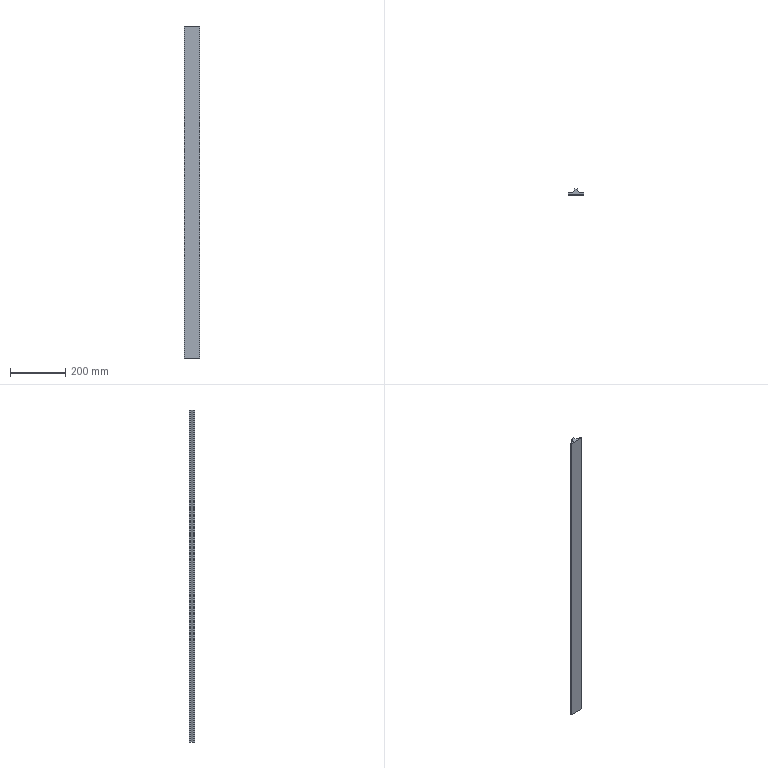Part | STEP file | SOPORTE RIEL 25mm | 1 solid | 13 faces | box 55 x 21.275 x 1200 mm | volume 648615 mm3 | plane 13
STEP:
#1=CARTESIAN_POINT('',(27.5,0.,-600.));
#2=VERTEX_POINT('',#1);
#3=CARTESIAN_POINT('',(27.5,6.,-600.));
#4=VERTEX_POINT('',#3);
#5=CARTESIAN_POINT('',(27.5,0.,-600.));
#6=DIRECTION('',(0.,1.,0.));
#7=VECTOR('',#6,1000.);
#8=LINE('',#5,#7);
#9=EDGE_CURVE('',#2,#4,#8,.T.);
#10=ORIENTED_EDGE('',*,*,#9,.T.);
#11=CARTESIAN_POINT('',(27.5,6.,600.));
#12=VERTEX_POINT('',#11);
#13=CARTESIAN_POINT('',(27.5,6.,600.));
#14=DIRECTION('',(0.,0.,-1.));
#15=VECTOR('',#14,1000.);
#16=LINE('',#13,#15);
#17=EDGE_CURVE('',#12,#4,#16,.T.);
#18=ORIENTED_EDGE('',*,*,#17,.F.);
#19=CARTESIAN_POINT('',(27.5,0.,600.));
#20=VERTEX_POINT('',#19);
#21=CARTESIAN_POINT('',(27.5,0.,600.));
#22=DIRECTION('',(0.,1.,0.));
#23=VECTOR('',#22,1000.);
#24=LINE('',#21,#23);
#25=EDGE_CURVE('',#20,#12,#24,.T.);
#26=ORIENTED_EDGE('',*,*,#25,.F.);
#27=CARTESIAN_POINT('',(27.5,0.,600.));
#28=DIRECTION('',(0.,0.,-1.));
#29=VECTOR('',#28,1000.);
#30=LINE('',#27,#29);
#31=EDGE_CURVE('',#20,#2,#30,.T.);
#32=ORIENTED_EDGE('',*,*,#31,.T.);
#33=EDGE_LOOP('',(#10,#18,#26,#32));
#34=FACE_OUTER_BOUND('',#33,.T.);
#35=CARTESIAN_POINT('',(27.5,0.,600.));
#36=DIRECTION('',(-1.,0.,0.));
#37=DIRECTION('',(0.,0.,1.));
#38=AXIS2_PLACEMENT_3D('',#35,#36,#37);
#39=PLANE('',#38);
#40=ADVANCED_FACE('',(#34),#39,.F.);
#41=CARTESIAN_POINT('',(11.,6.,-600.));
#42=VERTEX_POINT('',#41);
#43=CARTESIAN_POINT('',(27.5,6.,-600.));
#44=DIRECTION('',(-1.,0.,0.));
#45=VECTOR('',#44,1000.);
#46=LINE('',#43,#45);
#47=EDGE_CURVE('',#4,#42,#46,.T.);
#48=ORIENTED_EDGE('',*,*,#47,.T.);
#49=CARTESIAN_POINT('',(11.,6.,600.));
#50=VERTEX_POINT('',#49);
#51=CARTESIAN_POINT('',(11.,6.,600.));
#52=DIRECTION('',(0.,0.,-1.));
#53=VECTOR('',#52,1000.);
#54=LINE('',#51,#53);
#55=EDGE_CURVE('',#50,#42,#54,.T.);
#56=ORIENTED_EDGE('',*,*,#55,.F.);
#57=CARTESIAN_POINT('',(27.5,6.,600.));
#58=DIRECTION('',(-1.,0.,0.));
#59=VECTOR('',#58,1000.);
#60=LINE('',#57,#59);
#61=EDGE_CURVE('',#12,#50,#60,.T.);
#62=ORIENTED_EDGE('',*,*,#61,.F.);
#63=ORIENTED_EDGE('',*,*,#17,.T.);
#64=EDGE_LOOP('',(#48,#56,#62,#63));
#65=FACE_OUTER_BOUND('',#64,.T.);
#66=CARTESIAN_POINT('',(27.5,6.,600.));
#67=DIRECTION('',(0.,-1.,0.));
#68=DIRECTION('',(0.,0.,-1.));
#69=AXIS2_PLACEMENT_3D('',#66,#67,#68);
#70=PLANE('',#69);
#71=ADVANCED_FACE('',(#65),#70,.F.);
#72=CARTESIAN_POINT('',(5.5,15.,-600.));
#73=VERTEX_POINT('',#72);
#74=CARTESIAN_POINT('',(11.,6.,-600.));
#75=DIRECTION('',(-0.5215,0.8533,0.));
#76=VECTOR('',#75,1000.);
#77=LINE('',#74,#76);
#78=EDGE_CURVE('',#42,#73,#77,.T.);
#79=ORIENTED_EDGE('',*,*,#78,.T.);
#80=CARTESIAN_POINT('',(5.5,15.,600.));
#81=VERTEX_POINT('',#80);
#82=CARTESIAN_POINT('',(5.5,15.,600.));
#83=DIRECTION('',(0.,0.,-1.));
#84=VECTOR('',#83,1000.);
#85=LINE('',#82,#84);
#86=EDGE_CURVE('',#81,#73,#85,.T.);
#87=ORIENTED_EDGE('',*,*,#86,.F.);
#88=CARTESIAN_POINT('',(11.,6.,600.));
#89=DIRECTION('',(-0.5215,0.8533,0.));
#90=VECTOR('',#89,1000.);
#91=LINE('',#88,#90);
#92=EDGE_CURVE('',#50,#81,#91,.T.);
#93=ORIENTED_EDGE('',*,*,#92,.F.);
#94=ORIENTED_EDGE('',*,*,#55,.T.);
#95=EDGE_LOOP('',(#79,#87,#93,#94));
#96=FACE_OUTER_BOUND('',#95,.T.);
#97=CARTESIAN_POINT('',(11.,6.,600.));
#98=DIRECTION('',(-0.8533,-0.5215,0.));
#99=DIRECTION('',(0.5215,-0.8533,0.));
#100=AXIS2_PLACEMENT_3D('',#97,#98,#99);
#101=PLANE('',#100);
#102=ADVANCED_FACE('',(#96),#101,.F.);
#103=CARTESIAN_POINT('',(5.5,21.275,-600.));
#104=VERTEX_POINT('',#103);
#105=CARTESIAN_POINT('',(5.5,15.,-600.));
#106=DIRECTION('',(0.,1.,0.));
#107=VECTOR('',#106,1000.);
#108=LINE('',#105,#107);
#109=EDGE_CURVE('',#73,#104,#108,.T.);
#110=ORIENTED_EDGE('',*,*,#109,.T.);
#111=CARTESIAN_POINT('',(5.5,21.275,600.));
#112=VERTEX_POINT('',#111);
#113=CARTESIAN_POINT('',(5.5,21.275,600.));
#114=DIRECTION('',(0.,0.,-1.));
#115=VECTOR('',#114,1000.);
#116=LINE('',#113,#115);
#117=EDGE_CURVE('',#112,#104,#116,.T.);
#118=ORIENTED_EDGE('',*,*,#117,.F.);
#119=CARTESIAN_POINT('',(5.5,15.,600.));
#120=DIRECTION('',(0.,1.,0.));
#121=VECTOR('',#120,1000.);
#122=LINE('',#119,#121);
#123=EDGE_CURVE('',#81,#112,#122,.T.);
#124=ORIENTED_EDGE('',*,*,#123,.F.);
#125=ORIENTED_EDGE('',*,*,#86,.T.);
#126=EDGE_LOOP('',(#110,#118,#124,#125));
#127=FACE_OUTER_BOUND('',#126,.T.);
#128=CARTESIAN_POINT('',(5.5,15.,600.));
#129=DIRECTION('',(-1.,0.,0.));
#130=DIRECTION('',(0.,-1.,0.));
#131=AXIS2_PLACEMENT_3D('',#128,#129,#130);
#132=PLANE('',#131);
#133=ADVANCED_FACE('',(#127),#132,.F.);
#134=CARTESIAN_POINT('',(0.,20.,-600.));
#135=VERTEX_POINT('',#134);
#136=CARTESIAN_POINT('',(0.,20.,-600.));
#137=DIRECTION('',(-0.9742,-0.2258,0.));
#138=VECTOR('',#137,1000.);
#139=LINE('',#136,#138);
#140=EDGE_CURVE('',#104,#135,#139,.T.);
#141=ORIENTED_EDGE('',*,*,#140,.T.);
#142=CARTESIAN_POINT('',(0.,20.,600.));
#143=VERTEX_POINT('',#142);
#144=CARTESIAN_POINT('',(0.,20.,600.));
#145=DIRECTION('',(0.,0.,-1.));
#146=VECTOR('',#145,1000.);
#147=LINE('',#144,#146);
#148=EDGE_CURVE('',#143,#135,#147,.T.);
#149=ORIENTED_EDGE('',*,*,#148,.F.);
#150=CARTESIAN_POINT('',(0.,20.,600.));
#151=DIRECTION('',(-0.9742,-0.2258,0.));
#152=VECTOR('',#151,1000.);
#153=LINE('',#150,#152);
#154=EDGE_CURVE('',#112,#143,#153,.T.);
#155=ORIENTED_EDGE('',*,*,#154,.F.);
#156=ORIENTED_EDGE('',*,*,#117,.T.);
#157=EDGE_LOOP('',(#141,#149,#155,#156));
#158=FACE_OUTER_BOUND('',#157,.T.);
#159=CARTESIAN_POINT('',(0.,20.,600.));
#160=DIRECTION('',(0.2258,-0.9742,0.));
#161=DIRECTION('',(0.9742,0.2258,0.));
#162=AXIS2_PLACEMENT_3D('',#159,#160,#161);
#163=PLANE('',#162);
#164=ADVANCED_FACE('',(#158),#163,.F.);
#165=CARTESIAN_POINT('',(-5.5,21.275,-600.));
#166=VERTEX_POINT('',#165);
#167=CARTESIAN_POINT('',(-5.5,21.275,-600.));
#168=DIRECTION('',(-0.9742,0.2258,0.));
#169=VECTOR('',#168,1000.);
#170=LINE('',#167,#169);
#171=EDGE_CURVE('',#135,#166,#170,.T.);
#172=ORIENTED_EDGE('',*,*,#171,.T.);
#173=CARTESIAN_POINT('',(-5.5,21.275,600.));
#174=VERTEX_POINT('',#173);
#175=CARTESIAN_POINT('',(-5.5,21.275,600.));
#176=DIRECTION('',(0.,0.,-1.));
#177=VECTOR('',#176,1000.);
#178=LINE('',#175,#177);
#179=EDGE_CURVE('',#174,#166,#178,.T.);
#180=ORIENTED_EDGE('',*,*,#179,.F.);
#181=CARTESIAN_POINT('',(-5.5,21.275,600.));
#182=DIRECTION('',(-0.9742,0.2258,0.));
#183=VECTOR('',#182,1000.);
#184=LINE('',#181,#183);
#185=EDGE_CURVE('',#143,#174,#184,.T.);
#186=ORIENTED_EDGE('',*,*,#185,.F.);
#187=ORIENTED_EDGE('',*,*,#148,.T.);
#188=EDGE_LOOP('',(#172,#180,#186,#187));
#189=FACE_OUTER_BOUND('',#188,.T.);
#190=CARTESIAN_POINT('',(-5.5,21.275,600.));
#191=DIRECTION('',(-0.2258,-0.9742,0.));
#192=DIRECTION('',(0.9742,-0.2258,0.));
#193=AXIS2_PLACEMENT_3D('',#190,#191,#192);
#194=PLANE('',#193);
#195=ADVANCED_FACE('',(#189),#194,.F.);
#196=CARTESIAN_POINT('',(-5.5,15.,-600.));
#197=VERTEX_POINT('',#196);
#198=CARTESIAN_POINT('',(-5.5,15.,-600.));
#199=DIRECTION('',(0.,-1.,0.));
#200=VECTOR('',#199,1000.);
#201=LINE('',#198,#200);
#202=EDGE_CURVE('',#166,#197,#201,.T.);
#203=ORIENTED_EDGE('',*,*,#202,.T.);
#204=CARTESIAN_POINT('',(-5.5,15.,600.));
#205=VERTEX_POINT('',#204);
#206=CARTESIAN_POINT('',(-5.5,15.,600.));
#207=DIRECTION('',(0.,0.,-1.));
#208=VECTOR('',#207,1000.);
#209=LINE('',#206,#208);
#210=EDGE_CURVE('',#205,#197,#209,.T.);
#211=ORIENTED_EDGE('',*,*,#210,.F.);
#212=CARTESIAN_POINT('',(-5.5,15.,600.));
#213=DIRECTION('',(0.,-1.,0.));
#214=VECTOR('',#213,1000.);
#215=LINE('',#212,#214);
#216=EDGE_CURVE('',#174,#205,#215,.T.);
#217=ORIENTED_EDGE('',*,*,#216,.F.);
#218=ORIENTED_EDGE('',*,*,#179,.T.);
#219=EDGE_LOOP('',(#203,#211,#217,#218));
#220=FACE_OUTER_BOUND('',#219,.T.);
#221=CARTESIAN_POINT('',(-5.5,15.,600.));
#222=DIRECTION('',(1.,0.,0.));
#223=DIRECTION('',(0.,1.,0.));
#224=AXIS2_PLACEMENT_3D('',#221,#222,#223);
#225=PLANE('',#224);
#226=ADVANCED_FACE('',(#220),#225,.F.);
#227=CARTESIAN_POINT('',(-11.,6.,-600.));
#228=VERTEX_POINT('',#227);
#229=CARTESIAN_POINT('',(-11.,6.,-600.));
#230=DIRECTION('',(-0.5215,-0.8533,0.));
#231=VECTOR('',#230,1000.);
#232=LINE('',#229,#231);
#233=EDGE_CURVE('',#197,#228,#232,.T.);
#234=ORIENTED_EDGE('',*,*,#233,.T.);
#235=CARTESIAN_POINT('',(-11.,6.,600.));
#236=VERTEX_POINT('',#235);
#237=CARTESIAN_POINT('',(-11.,6.,600.));
#238=DIRECTION('',(0.,0.,-1.));
#239=VECTOR('',#238,1000.);
#240=LINE('',#237,#239);
#241=EDGE_CURVE('',#236,#228,#240,.T.);
#242=ORIENTED_EDGE('',*,*,#241,.F.);
#243=CARTESIAN_POINT('',(-11.,6.,600.));
#244=DIRECTION('',(-0.5215,-0.8533,0.));
#245=VECTOR('',#244,1000.);
#246=LINE('',#243,#245);
#247=EDGE_CURVE('',#205,#236,#246,.T.);
#248=ORIENTED_EDGE('',*,*,#247,.F.);
#249=ORIENTED_EDGE('',*,*,#210,.T.);
#250=EDGE_LOOP('',(#234,#242,#248,#249));
#251=FACE_OUTER_BOUND('',#250,.T.);
#252=CARTESIAN_POINT('',(-11.,6.,600.));
#253=DIRECTION('',(0.8533,-0.5215,0.));
#254=DIRECTION('',(0.5215,0.8533,0.));
#255=AXIS2_PLACEMENT_3D('',#252,#253,#254);
#256=PLANE('',#255);
#257=ADVANCED_FACE('',(#251),#256,.F.);
#258=CARTESIAN_POINT('',(-27.5,6.,-600.));
#259=VERTEX_POINT('',#258);
#260=CARTESIAN_POINT('',(-27.5,6.,-600.));
#261=DIRECTION('',(-1.,0.,0.));
#262=VECTOR('',#261,1000.);
#263=LINE('',#260,#262);
#264=EDGE_CURVE('',#228,#259,#263,.T.);
#265=ORIENTED_EDGE('',*,*,#264,.T.);
#266=CARTESIAN_POINT('',(-27.5,6.,600.));
#267=VERTEX_POINT('',#266);
#268=CARTESIAN_POINT('',(-27.5,6.,600.));
#269=DIRECTION('',(0.,0.,-1.));
#270=VECTOR('',#269,1000.);
#271=LINE('',#268,#270);
#272=EDGE_CURVE('',#267,#259,#271,.T.);
#273=ORIENTED_EDGE('',*,*,#272,.F.);
#274=CARTESIAN_POINT('',(-27.5,6.,600.));
#275=DIRECTION('',(-1.,0.,0.));
#276=VECTOR('',#275,1000.);
#277=LINE('',#274,#276);
#278=EDGE_CURVE('',#236,#267,#277,.T.);
#279=ORIENTED_EDGE('',*,*,#278,.F.);
#280=ORIENTED_EDGE('',*,*,#241,.T.);
#281=EDGE_LOOP('',(#265,#273,#279,#280));
#282=FACE_OUTER_BOUND('',#281,.T.);
#283=CARTESIAN_POINT('',(-27.5,6.,600.));
#284=DIRECTION('',(0.,-1.,0.));
#285=DIRECTION('',(0.,0.,-1.));
#286=AXIS2_PLACEMENT_3D('',#283,#284,#285);
#287=PLANE('',#286);
#288=ADVANCED_FACE('',(#282),#287,.F.);
#289=CARTESIAN_POINT('',(-27.5,0.,-600.));
#290=VERTEX_POINT('',#289);
#291=CARTESIAN_POINT('',(-27.5,0.,-600.));
#292=DIRECTION('',(0.,-1.,0.));
#293=VECTOR('',#292,1000.);
#294=LINE('',#291,#293);
#295=EDGE_CURVE('',#259,#290,#294,.T.);
#296=ORIENTED_EDGE('',*,*,#295,.T.);
#297=CARTESIAN_POINT('',(-27.5,0.,600.));
#298=VERTEX_POINT('',#297);
#299=CARTESIAN_POINT('',(-27.5,0.,600.));
#300=DIRECTION('',(0.,0.,-1.));
#301=VECTOR('',#300,1000.);
#302=LINE('',#299,#301);
#303=EDGE_CURVE('',#298,#290,#302,.T.);
#304=ORIENTED_EDGE('',*,*,#303,.F.);
#305=CARTESIAN_POINT('',(-27.5,0.,600.));
#306=DIRECTION('',(0.,-1.,0.));
#307=VECTOR('',#306,1000.);
#308=LINE('',#305,#307);
#309=EDGE_CURVE('',#267,#298,#308,.T.);
#310=ORIENTED_EDGE('',*,*,#309,.F.);
#311=ORIENTED_EDGE('',*,*,#272,.T.);
#312=EDGE_LOOP('',(#296,#304,#310,#311));
#313=FACE_OUTER_BOUND('',#312,.T.);
#314=CARTESIAN_POINT('',(-27.5,0.,600.));
#315=DIRECTION('',(1.,0.,0.));
#316=DIRECTION('',(0.,0.,-1.));
#317=AXIS2_PLACEMENT_3D('',#314,#315,#316);
#318=PLANE('',#317);
#319=ADVANCED_FACE('',(#313),#318,.F.);
#320=CARTESIAN_POINT('',(-27.5,0.,-600.));
#321=DIRECTION('',(1.,0.,0.));
#322=VECTOR('',#321,1000.);
#323=LINE('',#320,#322);
#324=EDGE_CURVE('',#290,#2,#323,.T.);
#325=ORIENTED_EDGE('',*,*,#324,.T.);
#326=ORIENTED_EDGE('',*,*,#31,.F.);
#327=CARTESIAN_POINT('',(-27.5,0.,600.));
#328=DIRECTION('',(1.,0.,0.));
#329=VECTOR('',#328,1000.);
#330=LINE('',#327,#329);
#331=EDGE_CURVE('',#298,#20,#330,.T.);
#332=ORIENTED_EDGE('',*,*,#331,.F.);
#333=ORIENTED_EDGE('',*,*,#303,.T.);
#334=EDGE_LOOP('',(#325,#326,#332,#333));
#335=FACE_OUTER_BOUND('',#334,.T.);
#336=CARTESIAN_POINT('',(-27.5,0.,600.));
#337=DIRECTION('',(0.,1.,0.));
#338=DIRECTION('',(0.,0.,1.));
#339=AXIS2_PLACEMENT_3D('',#336,#337,#338);
#340=PLANE('',#339);
#341=ADVANCED_FACE('',(#335),#340,.F.);
#342=ORIENTED_EDGE('',*,*,#25,.T.);
#343=ORIENTED_EDGE('',*,*,#61,.T.);
#344=ORIENTED_EDGE('',*,*,#92,.T.);
#345=ORIENTED_EDGE('',*,*,#123,.T.);
#346=ORIENTED_EDGE('',*,*,#154,.T.);
#347=ORIENTED_EDGE('',*,*,#185,.T.);
#348=ORIENTED_EDGE('',*,*,#216,.T.);
#349=ORIENTED_EDGE('',*,*,#247,.T.);
#350=ORIENTED_EDGE('',*,*,#278,.T.);
#351=ORIENTED_EDGE('',*,*,#309,.T.);
#352=ORIENTED_EDGE('',*,*,#331,.T.);
#353=EDGE_LOOP('',(#342,#343,#344,#345,#346,#347,#348,#349,#350,#351,#352));
#354=FACE_OUTER_BOUND('',#353,.T.);
#355=CARTESIAN_POINT('',(0.,0.,600.));
#356=DIRECTION('',(0.,0.,1.));
#357=DIRECTION('',(1.,0.,0.));
#358=AXIS2_PLACEMENT_3D('',#355,#356,#357);
#359=PLANE('',#358);
#360=ADVANCED_FACE('',(#354),#359,.T.);
#361=ORIENTED_EDGE('',*,*,#9,.F.);
#362=ORIENTED_EDGE('',*,*,#324,.F.);
#363=ORIENTED_EDGE('',*,*,#295,.F.);
#364=ORIENTED_EDGE('',*,*,#264,.F.);
#365=ORIENTED_EDGE('',*,*,#233,.F.);
#366=ORIENTED_EDGE('',*,*,#202,.F.);
#367=ORIENTED_EDGE('',*,*,#171,.F.);
#368=ORIENTED_EDGE('',*,*,#140,.F.);
#369=ORIENTED_EDGE('',*,*,#109,.F.);
#370=ORIENTED_EDGE('',*,*,#78,.F.);
#371=ORIENTED_EDGE('',*,*,#47,.F.);
#372=EDGE_LOOP('',(#361,#362,#363,#364,#365,#366,#367,#368,#369,#370,#371));
#373=FACE_OUTER_BOUND('',#372,.T.);
#374=CARTESIAN_POINT('',(0.,0.,-600.));
#375=DIRECTION('',(0.,0.,1.));
#376=DIRECTION('',(1.,0.,0.));
#377=AXIS2_PLACEMENT_3D('',#374,#375,#376);
#378=PLANE('',#377);
#379=ADVANCED_FACE('',(#373),#378,.F.);
#380=CLOSED_SHELL('',(#40,#71,#102,#133,#164,#195,#226,#257,#288,#319,#341,#360,#379));
#381=MANIFOLD_SOLID_BREP('',#380);
#382=CARTESIAN_POINT('',(0.,0.,0.));
#383=DIRECTION('',(0.,0.,1.));
#384=DIRECTION('',(1.,0.,0.));
#385=AXIS2_PLACEMENT_3D('',#382,#383,#384);
#386=(LENGTH_UNIT()NAMED_UNIT(*)SI_UNIT(.MILLI.,.METRE.));
#387=UNCERTAINTY_MEASURE_WITH_UNIT(LENGTH_MEASURE(0.00001),#386,'','');
#388=(NAMED_UNIT(*)PLANE_ANGLE_UNIT()SI_UNIT($,.RADIAN.));
#389=(NAMED_UNIT(*)SI_UNIT($,.STERADIAN.)SOLID_ANGLE_UNIT());
#390=(GEOMETRIC_REPRESENTATION_CONTEXT(3)GLOBAL_UNCERTAINTY_ASSIGNED_CONTEXT((#387))GLOBAL_UNIT_ASSIGNED_CONTEXT((#386,#388,#389))REPRESENTATION_CONTEXT('',''));
#391=ADVANCED_BREP_SHAPE_REPRESENTATION('',(#381,#385),#390);